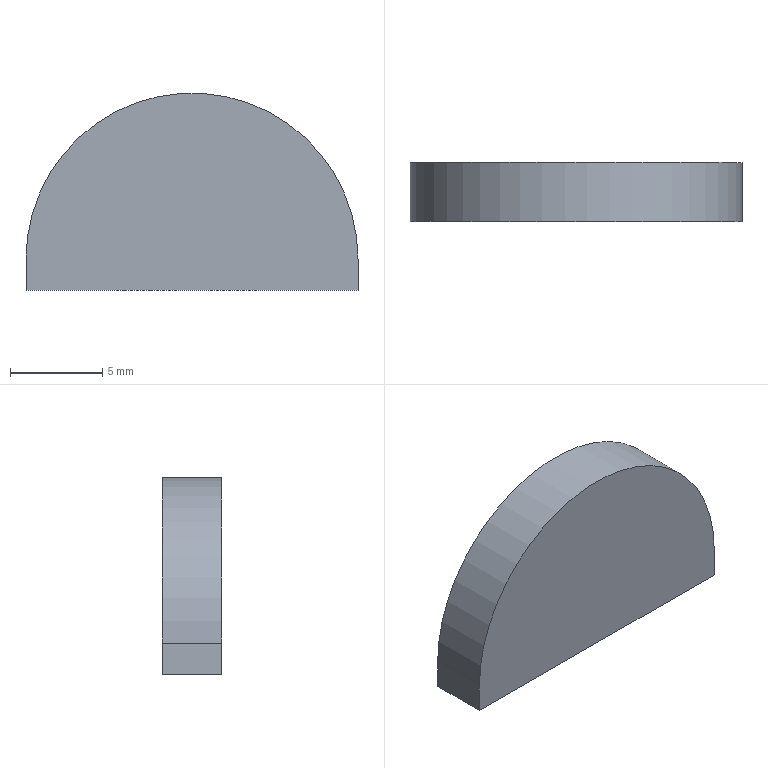Part | SolidWorks | features Extrusion 1 | 1 solid | 6 faces | box 18 x 3.2 x 10.7 mm | volume 505.07 mm3 | plane 5 | cylinder 1 | commonest cylinder face diameters 18 x1
STEP:
#1=CARTESIAN_POINT('',(-27.129,0.,0.));
#2=VERTEX_POINT('',#1);
#3=CARTESIAN_POINT('',(-9.129,0.,0.));
#4=VERTEX_POINT('',#3);
#5=CARTESIAN_POINT('',(-18.129,0.,0.));
#6=DIRECTION('',(0.,1.,0.));
#7=DIRECTION('',(0.,0.,1.));
#8=AXIS2_PLACEMENT_3D('',#5,#6,#7);
#9=CIRCLE('',#8,9.);
#10=EDGE_CURVE('',#2,#4,#9,.T.);
#11=ORIENTED_EDGE('',*,*,#10,.T.);
#12=CARTESIAN_POINT('',(-9.129,3.2,0.));
#13=VERTEX_POINT('',#12);
#14=CARTESIAN_POINT('',(-9.129,3.2,0.));
#15=DIRECTION('',(0.,-1.,0.));
#16=VECTOR('',#15,1000.);
#17=LINE('',#14,#16);
#18=EDGE_CURVE('',#13,#4,#17,.T.);
#19=ORIENTED_EDGE('',*,*,#18,.F.);
#20=CARTESIAN_POINT('',(-27.129,3.2,0.));
#21=VERTEX_POINT('',#20);
#22=CARTESIAN_POINT('',(-18.129,3.2,0.));
#23=DIRECTION('',(0.,1.,0.));
#24=DIRECTION('',(0.,0.,1.));
#25=AXIS2_PLACEMENT_3D('',#22,#23,#24);
#26=CIRCLE('',#25,9.);
#27=EDGE_CURVE('',#21,#13,#26,.T.);
#28=ORIENTED_EDGE('',*,*,#27,.F.);
#29=CARTESIAN_POINT('',(-27.129,3.2,0.));
#30=DIRECTION('',(0.,-1.,0.));
#31=VECTOR('',#30,1000.);
#32=LINE('',#29,#31);
#33=EDGE_CURVE('',#21,#2,#32,.T.);
#34=ORIENTED_EDGE('',*,*,#33,.T.);
#35=EDGE_LOOP('',(#11,#19,#28,#34));
#36=FACE_OUTER_BOUND('',#35,.T.);
#37=CARTESIAN_POINT('',(-18.129,3.2,0.));
#38=DIRECTION('',(0.,-1.,0.));
#39=DIRECTION('',(0.,0.,-1.));
#40=AXIS2_PLACEMENT_3D('',#37,#38,#39);
#41=CYLINDRICAL_SURFACE('',#40,9.);
#42=ADVANCED_FACE('',(#36),#41,.T.);
#43=CARTESIAN_POINT('',(-9.129,0.,-1.7));
#44=VERTEX_POINT('',#43);
#45=CARTESIAN_POINT('',(-9.129,0.,-1.7));
#46=DIRECTION('',(0.,0.,-1.));
#47=VECTOR('',#46,1000.);
#48=LINE('',#45,#47);
#49=EDGE_CURVE('',#4,#44,#48,.T.);
#50=ORIENTED_EDGE('',*,*,#49,.T.);
#51=CARTESIAN_POINT('',(-9.129,3.2,-1.7));
#52=VERTEX_POINT('',#51);
#53=CARTESIAN_POINT('',(-9.129,3.2,-1.7));
#54=DIRECTION('',(0.,-1.,0.));
#55=VECTOR('',#54,1000.);
#56=LINE('',#53,#55);
#57=EDGE_CURVE('',#52,#44,#56,.T.);
#58=ORIENTED_EDGE('',*,*,#57,.F.);
#59=CARTESIAN_POINT('',(-9.129,3.2,-1.7));
#60=DIRECTION('',(0.,0.,-1.));
#61=VECTOR('',#60,1000.);
#62=LINE('',#59,#61);
#63=EDGE_CURVE('',#13,#52,#62,.T.);
#64=ORIENTED_EDGE('',*,*,#63,.F.);
#65=ORIENTED_EDGE('',*,*,#18,.T.);
#66=EDGE_LOOP('',(#50,#58,#64,#65));
#67=FACE_OUTER_BOUND('',#66,.T.);
#68=CARTESIAN_POINT('',(-9.129,3.2,-1.7));
#69=DIRECTION('',(-1.,0.,0.));
#70=DIRECTION('',(0.,0.,1.));
#71=AXIS2_PLACEMENT_3D('',#68,#69,#70);
#72=PLANE('',#71);
#73=ADVANCED_FACE('',(#67),#72,.F.);
#74=CARTESIAN_POINT('',(-27.129,0.,-1.7));
#75=VERTEX_POINT('',#74);
#76=CARTESIAN_POINT('',(-27.129,0.,-1.7));
#77=DIRECTION('',(-1.,0.,0.));
#78=VECTOR('',#77,1000.);
#79=LINE('',#76,#78);
#80=EDGE_CURVE('',#44,#75,#79,.T.);
#81=ORIENTED_EDGE('',*,*,#80,.T.);
#82=CARTESIAN_POINT('',(-27.129,3.2,-1.7));
#83=VERTEX_POINT('',#82);
#84=CARTESIAN_POINT('',(-27.129,3.2,-1.7));
#85=DIRECTION('',(0.,-1.,0.));
#86=VECTOR('',#85,1000.);
#87=LINE('',#84,#86);
#88=EDGE_CURVE('',#83,#75,#87,.T.);
#89=ORIENTED_EDGE('',*,*,#88,.F.);
#90=CARTESIAN_POINT('',(-27.129,3.2,-1.7));
#91=DIRECTION('',(-1.,0.,0.));
#92=VECTOR('',#91,1000.);
#93=LINE('',#90,#92);
#94=EDGE_CURVE('',#52,#83,#93,.T.);
#95=ORIENTED_EDGE('',*,*,#94,.F.);
#96=ORIENTED_EDGE('',*,*,#57,.T.);
#97=EDGE_LOOP('',(#81,#89,#95,#96));
#98=FACE_OUTER_BOUND('',#97,.T.);
#99=CARTESIAN_POINT('',(-27.129,3.2,-1.7));
#100=DIRECTION('',(0.,0.,1.));
#101=DIRECTION('',(1.,0.,0.));
#102=AXIS2_PLACEMENT_3D('',#99,#100,#101);
#103=PLANE('',#102);
#104=ADVANCED_FACE('',(#98),#103,.F.);
#105=CARTESIAN_POINT('',(-27.129,0.,0.));
#106=DIRECTION('',(0.,0.,1.));
#107=VECTOR('',#106,1000.);
#108=LINE('',#105,#107);
#109=EDGE_CURVE('',#75,#2,#108,.T.);
#110=ORIENTED_EDGE('',*,*,#109,.T.);
#111=ORIENTED_EDGE('',*,*,#33,.F.);
#112=CARTESIAN_POINT('',(-27.129,3.2,0.));
#113=DIRECTION('',(0.,0.,1.));
#114=VECTOR('',#113,1000.);
#115=LINE('',#112,#114);
#116=EDGE_CURVE('',#83,#21,#115,.T.);
#117=ORIENTED_EDGE('',*,*,#116,.F.);
#118=ORIENTED_EDGE('',*,*,#88,.T.);
#119=EDGE_LOOP('',(#110,#111,#117,#118));
#120=FACE_OUTER_BOUND('',#119,.T.);
#121=CARTESIAN_POINT('',(-27.129,3.2,0.));
#122=DIRECTION('',(1.,0.,0.));
#123=DIRECTION('',(0.,0.,-1.));
#124=AXIS2_PLACEMENT_3D('',#121,#122,#123);
#125=PLANE('',#124);
#126=ADVANCED_FACE('',(#120),#125,.F.);
#127=ORIENTED_EDGE('',*,*,#27,.T.);
#128=ORIENTED_EDGE('',*,*,#63,.T.);
#129=ORIENTED_EDGE('',*,*,#94,.T.);
#130=ORIENTED_EDGE('',*,*,#116,.T.);
#131=EDGE_LOOP('',(#127,#128,#129,#130));
#132=FACE_OUTER_BOUND('',#131,.T.);
#133=CARTESIAN_POINT('',(-18.129,3.2,0.));
#134=DIRECTION('',(0.,1.,0.));
#135=DIRECTION('',(0.,0.,1.));
#136=AXIS2_PLACEMENT_3D('',#133,#134,#135);
#137=PLANE('',#136);
#138=ADVANCED_FACE('',(#132),#137,.T.);
#139=ORIENTED_EDGE('',*,*,#10,.F.);
#140=ORIENTED_EDGE('',*,*,#109,.F.);
#141=ORIENTED_EDGE('',*,*,#80,.F.);
#142=ORIENTED_EDGE('',*,*,#49,.F.);
#143=EDGE_LOOP('',(#139,#140,#141,#142));
#144=FACE_OUTER_BOUND('',#143,.T.);
#145=CARTESIAN_POINT('',(-18.129,0.,0.));
#146=DIRECTION('',(0.,1.,0.));
#147=DIRECTION('',(0.,0.,1.));
#148=AXIS2_PLACEMENT_3D('',#145,#146,#147);
#149=PLANE('',#148);
#150=ADVANCED_FACE('',(#144),#149,.F.);
#151=CLOSED_SHELL('',(#42,#73,#104,#126,#138,#150));
#152=MANIFOLD_SOLID_BREP('',#151);
#153=CARTESIAN_POINT('',(0.,0.,0.));
#154=DIRECTION('',(0.,0.,1.));
#155=DIRECTION('',(1.,0.,0.));
#156=AXIS2_PLACEMENT_3D('',#153,#154,#155);
#157=(LENGTH_UNIT()NAMED_UNIT(*)SI_UNIT(.MILLI.,.METRE.));
#158=UNCERTAINTY_MEASURE_WITH_UNIT(LENGTH_MEASURE(0.00001),#157,'','');
#159=(NAMED_UNIT(*)PLANE_ANGLE_UNIT()SI_UNIT($,.RADIAN.));
#160=(NAMED_UNIT(*)SI_UNIT($,.STERADIAN.)SOLID_ANGLE_UNIT());
#161=(GEOMETRIC_REPRESENTATION_CONTEXT(3)GLOBAL_UNCERTAINTY_ASSIGNED_CONTEXT((#158))GLOBAL_UNIT_ASSIGNED_CONTEXT((#157,#159,#160))REPRESENTATION_CONTEXT('',''));
#162=ADVANCED_BREP_SHAPE_REPRESENTATION('',(#152,#156),#161);